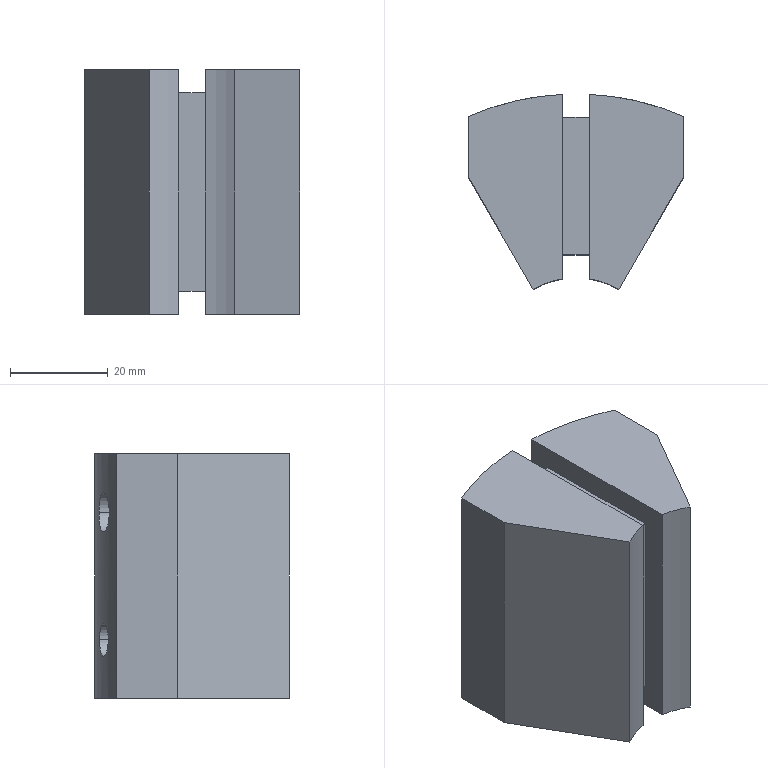Part | SolidWorks | features 3DProfileFeature 2, HoleWzd 2, Extrusion 1, ICE 1 | 1 solid | 34 faces | box 44 x 39.776 x 50 mm | volume 60767 mm3 | plane 14 | cylinder 12 | cone 8 | commonest cylinder face diameters 6.8 x4 8 x4 35 x2 110 x2
STEP:
#1=CARTESIAN_POINT('',(-9.048,33.766,-13.));
#2=VERTEX_POINT('',#1);
#3=CARTESIAN_POINT('',(-12.86,34.859,-13.));
#4=VERTEX_POINT('',#3);
#5=CARTESIAN_POINT('',(-12.86,34.859,-13.));
#6=DIRECTION('',(-0.9613,0.2756,0.));
#7=VECTOR('',#6,1000.);
#8=LINE('',#5,#7);
#9=EDGE_CURVE('',#2,#4,#8,.T.);
#10=ORIENTED_EDGE('',*,*,#9,.F.);
#11=CARTESIAN_POINT('',(-6.292,36.619,-13.));
#12=VERTEX_POINT('',#11);
#13=CARTESIAN_POINT('',(-6.292,36.619,-13.));
#14=DIRECTION('',(0.6947,0.7193,0.));
#15=VECTOR('',#14,1000.);
#16=LINE('',#13,#15);
#17=EDGE_CURVE('',#2,#12,#16,.T.);
#18=ORIENTED_EDGE('',*,*,#17,.T.);
#19=CARTESIAN_POINT('',(-9.576,35.739,-13.));
#20=DIRECTION('',(-0.2588,0.9659,0.));
#21=DIRECTION('',(-0.9659,-0.2588,0.));
#22=AXIS2_PLACEMENT_3D('',#19,#20,#21);
#23=CIRCLE('',#22,3.4);
#24=EDGE_CURVE('',#12,#4,#23,.T.);
#25=ORIENTED_EDGE('',*,*,#24,.T.);
#26=EDGE_LOOP('',(#10,#18,#25));
#27=FACE_OUTER_BOUND('',#26,.T.);
#28=CARTESIAN_POINT('',(-9.576,35.739,-13.));
#29=DIRECTION('',(-0.2588,0.9659,0.));
#30=DIRECTION('',(-0.9659,-0.2588,0.));
#31=AXIS2_PLACEMENT_3D('',#28,#29,#30);
#32=CONICAL_SURFACE('',#31,3.4,1.03);
#33=ADVANCED_FACE('',(#27),#32,.F.);
#34=ORIENTED_EDGE('',*,*,#24,.F.);
#35=CARTESIAN_POINT('',(-10.924,53.904,-13.));
#36=VERTEX_POINT('',#35);
#37=CARTESIAN_POINT('',(-10.951,54.006,-13.));
#38=DIRECTION('',(-0.2588,0.9659,0.));
#39=VECTOR('',#38,1000.);
#40=LINE('',#37,#39);
#41=EDGE_CURVE('',#12,#36,#40,.T.);
#42=ORIENTED_EDGE('',*,*,#41,.T.);
#43=CARTESIAN_POINT('',(-17.492,52.144,-13.));
#44=VERTEX_POINT('',#43);
#45=CARTESIAN_POINT('',(-17.492,52.144,-13.));
#46=CARTESIAN_POINT('',(-17.492,52.144,-13.225));
#47=CARTESIAN_POINT('',(-17.471,52.151,-13.446));
#48=CARTESIAN_POINT('',(-17.389,52.179,-13.88));
#49=CARTESIAN_POINT('',(-17.327,52.2,-14.096));
#50=CARTESIAN_POINT('',(-17.164,52.253,-14.508));
#51=CARTESIAN_POINT('',(-17.065,52.286,-14.703));
#52=CARTESIAN_POINT('',(-16.83,52.362,-15.073));
#53=CARTESIAN_POINT('',(-16.693,52.406,-15.248));
#54=CARTESIAN_POINT('',(-16.394,52.5,-15.561));
#55=CARTESIAN_POINT('',(-16.23,52.551,-15.702));
#56=CARTESIAN_POINT('',(-15.874,52.66,-15.951));
#57=CARTESIAN_POINT('',(-15.685,52.717,-16.056));
#58=CARTESIAN_POINT('',(-15.292,52.832,-16.226));
#59=CARTESIAN_POINT('',(-15.086,52.891,-16.291));
#60=CARTESIAN_POINT('',(-14.663,53.01,-16.378));
#61=CARTESIAN_POINT('',(-14.45,53.068,-16.4));
#62=CARTESIAN_POINT('',(-14.022,53.183,-16.4));
#63=CARTESIAN_POINT('',(-13.804,53.24,-16.378));
#64=CARTESIAN_POINT('',(-13.381,53.348,-16.291));
#65=CARTESIAN_POINT('',(-13.176,53.399,-16.227));
#66=CARTESIAN_POINT('',(-12.775,53.496,-16.057));
#67=CARTESIAN_POINT('',(-12.582,53.542,-15.95));
#68=CARTESIAN_POINT('',(-12.222,53.625,-15.704));
#69=CARTESIAN_POINT('',(-12.055,53.663,-15.563));
#70=CARTESIAN_POINT('',(-11.745,53.732,-15.246));
#71=CARTESIAN_POINT('',(-11.607,53.761,-15.074));
#72=CARTESIAN_POINT('',(-11.366,53.813,-14.706));
#73=CARTESIAN_POINT('',(-11.261,53.835,-14.507));
#74=CARTESIAN_POINT('',(-11.094,53.87,-14.095));
#75=CARTESIAN_POINT('',(-11.031,53.882,-13.883));
#76=CARTESIAN_POINT('',(-10.946,53.9,-13.447));
#77=CARTESIAN_POINT('',(-10.924,53.904,-13.222));
#78=CARTESIAN_POINT('',(-10.924,53.904,-13.));
#79=B_SPLINE_CURVE_WITH_KNOTS('',3,(#45,#46,#47,#48,#49,#50,#51,#52,#53,#54,#55,#56,#57,#58,#59,#60,#61,#62,#63,#64,#65,#66,#67,#68,#69,#70,#71,#72,#73,#74,#75,#76,#77,#78),.UNSPECIFIED.,.F.,.F.,(4,2,2,2,2,2,2,2,2,2,2,2,2,2,2,2,4),(0.,0.0006645,0.001329,0.001994,0.002658,0.003323,0.003987,0.004652,0.005316,0.005981,0.006645,0.00731,0.007974,0.008639,0.009303,0.009968,0.01063),.UNSPECIFIED.);
#80=EDGE_CURVE('',#44,#36,#79,.T.);
#81=ORIENTED_EDGE('',*,*,#80,.F.);
#82=CARTESIAN_POINT('',(-17.519,52.246,-13.));
#83=DIRECTION('',(-0.2588,0.9659,0.));
#84=VECTOR('',#83,1000.);
#85=LINE('',#82,#84);
#86=EDGE_CURVE('',#4,#44,#85,.T.);
#87=ORIENTED_EDGE('',*,*,#86,.F.);
#88=EDGE_LOOP('',(#34,#42,#81,#87));
#89=FACE_OUTER_BOUND('',#88,.T.);
#90=CARTESIAN_POINT('',(-14.235,53.126,-13.));
#91=DIRECTION('',(-0.2588,0.9659,0.));
#92=DIRECTION('',(-0.9659,-0.2588,0.));
#93=AXIS2_PLACEMENT_3D('',#90,#91,#92);
#94=CYLINDRICAL_SURFACE('',#93,3.4);
#95=ADVANCED_FACE('',(#89),#94,.F.);
#96=CARTESIAN_POINT('',(9.048,33.766,13.));
#97=VERTEX_POINT('',#96);
#98=CARTESIAN_POINT('',(6.292,36.619,13.));
#99=VERTEX_POINT('',#98);
#100=CARTESIAN_POINT('',(6.292,36.619,13.));
#101=DIRECTION('',(-0.6947,0.7193,0.));
#102=VECTOR('',#101,1000.);
#103=LINE('',#100,#102);
#104=EDGE_CURVE('',#97,#99,#103,.T.);
#105=ORIENTED_EDGE('',*,*,#104,.F.);
#106=CARTESIAN_POINT('',(12.86,34.859,13.));
#107=VERTEX_POINT('',#106);
#108=CARTESIAN_POINT('',(12.86,34.859,13.));
#109=DIRECTION('',(0.9613,0.2756,0.));
#110=VECTOR('',#109,1000.);
#111=LINE('',#108,#110);
#112=EDGE_CURVE('',#97,#107,#111,.T.);
#113=ORIENTED_EDGE('',*,*,#112,.T.);
#114=CARTESIAN_POINT('',(9.576,35.739,13.));
#115=DIRECTION('',(0.2588,0.9659,0.));
#116=DIRECTION('',(-0.9659,0.2588,0.));
#117=AXIS2_PLACEMENT_3D('',#114,#115,#116);
#118=CIRCLE('',#117,3.4);
#119=EDGE_CURVE('',#107,#99,#118,.T.);
#120=ORIENTED_EDGE('',*,*,#119,.T.);
#121=EDGE_LOOP('',(#105,#113,#120));
#122=FACE_OUTER_BOUND('',#121,.T.);
#123=CARTESIAN_POINT('',(9.576,35.739,13.));
#124=DIRECTION('',(0.2588,0.9659,0.));
#125=DIRECTION('',(-0.9659,0.2588,0.));
#126=AXIS2_PLACEMENT_3D('',#123,#124,#125);
#127=CONICAL_SURFACE('',#126,3.4,1.03);
#128=ADVANCED_FACE('',(#122),#127,.F.);
#129=ORIENTED_EDGE('',*,*,#119,.F.);
#130=CARTESIAN_POINT('',(17.492,52.144,13.));
#131=VERTEX_POINT('',#130);
#132=CARTESIAN_POINT('',(17.519,52.246,13.));
#133=DIRECTION('',(0.2588,0.9659,0.));
#134=VECTOR('',#133,1000.);
#135=LINE('',#132,#134);
#136=EDGE_CURVE('',#107,#131,#135,.T.);
#137=ORIENTED_EDGE('',*,*,#136,.T.);
#138=CARTESIAN_POINT('',(10.924,53.904,13.));
#139=VERTEX_POINT('',#138);
#140=CARTESIAN_POINT('',(10.924,53.904,13.));
#141=CARTESIAN_POINT('',(10.924,53.904,12.775));
#142=CARTESIAN_POINT('',(10.945,53.9,12.554));
#143=CARTESIAN_POINT('',(11.03,53.883,12.12));
#144=CARTESIAN_POINT('',(11.094,53.869,11.904));
#145=CARTESIAN_POINT('',(11.262,53.835,11.492));
#146=CARTESIAN_POINT('',(11.364,53.813,11.297));
#147=CARTESIAN_POINT('',(11.606,53.762,10.927));
#148=CARTESIAN_POINT('',(11.746,53.731,10.752));
#149=CARTESIAN_POINT('',(12.053,53.663,10.439));
#150=CARTESIAN_POINT('',(12.22,53.626,10.298));
#151=CARTESIAN_POINT('',(12.582,53.542,10.049));
#152=CARTESIAN_POINT('',(12.775,53.496,9.944));
#153=CARTESIAN_POINT('',(13.173,53.4,9.774));
#154=CARTESIAN_POINT('',(13.381,53.348,9.709));
#155=CARTESIAN_POINT('',(13.806,53.239,9.622));
#156=CARTESIAN_POINT('',(14.02,53.184,9.6));
#157=CARTESIAN_POINT('',(14.448,53.069,9.6));
#158=CARTESIAN_POINT('',(14.665,53.009,9.622));
#159=CARTESIAN_POINT('',(15.085,52.891,9.709));
#160=CARTESIAN_POINT('',(15.289,52.833,9.773));
#161=CARTESIAN_POINT('',(15.684,52.717,9.943));
#162=CARTESIAN_POINT('',(15.875,52.659,10.05));
#163=CARTESIAN_POINT('',(16.228,52.552,10.296));
#164=CARTESIAN_POINT('',(16.392,52.501,10.437));
#165=CARTESIAN_POINT('',(16.695,52.405,10.754));
#166=CARTESIAN_POINT('',(16.829,52.362,10.926));
#167=CARTESIAN_POINT('',(17.064,52.286,11.294));
#168=CARTESIAN_POINT('',(17.165,52.253,11.493));
#169=CARTESIAN_POINT('',(17.327,52.199,11.905));
#170=CARTESIAN_POINT('',(17.388,52.179,12.117));
#171=CARTESIAN_POINT('',(17.471,52.151,12.553));
#172=CARTESIAN_POINT('',(17.492,52.144,12.778));
#173=CARTESIAN_POINT('',(17.492,52.144,13.));
#174=B_SPLINE_CURVE_WITH_KNOTS('',3,(#140,#141,#142,#143,#144,#145,#146,#147,#148,#149,#150,#151,#152,#153,#154,#155,#156,#157,#158,#159,#160,#161,#162,#163,#164,#165,#166,#167,#168,#169,#170,#171,#172,#173),.UNSPECIFIED.,.F.,.F.,(4,2,2,2,2,2,2,2,2,2,2,2,2,2,2,2,4),(0.,0.0006645,0.001329,0.001994,0.002658,0.003323,0.003987,0.004652,0.005316,0.005981,0.006645,0.00731,0.007974,0.008639,0.009303,0.009968,0.01063),.UNSPECIFIED.);
#175=EDGE_CURVE('',#139,#131,#174,.T.);
#176=ORIENTED_EDGE('',*,*,#175,.F.);
#177=CARTESIAN_POINT('',(10.951,54.006,13.));
#178=DIRECTION('',(0.2588,0.9659,0.));
#179=VECTOR('',#178,1000.);
#180=LINE('',#177,#179);
#181=EDGE_CURVE('',#99,#139,#180,.T.);
#182=ORIENTED_EDGE('',*,*,#181,.F.);
#183=EDGE_LOOP('',(#129,#137,#176,#182));
#184=FACE_OUTER_BOUND('',#183,.T.);
#185=CARTESIAN_POINT('',(14.235,53.126,13.));
#186=DIRECTION('',(0.2588,0.9659,0.));
#187=DIRECTION('',(-0.9659,0.2588,0.));
#188=AXIS2_PLACEMENT_3D('',#185,#186,#187);
#189=CYLINDRICAL_SURFACE('',#188,3.4);
#190=ADVANCED_FACE('',(#184),#189,.F.);
#191=CARTESIAN_POINT('',(-9.731,36.315,13.));
#192=VERTEX_POINT('',#191);
#193=CARTESIAN_POINT('',(-14.216,37.602,13.));
#194=VERTEX_POINT('',#193);
#195=CARTESIAN_POINT('',(-14.216,37.602,13.));
#196=DIRECTION('',(-0.9613,0.2756,0.));
#197=VECTOR('',#196,1000.);
#198=LINE('',#195,#197);
#199=EDGE_CURVE('',#192,#194,#198,.T.);
#200=ORIENTED_EDGE('',*,*,#199,.F.);
#201=CARTESIAN_POINT('',(-6.489,39.672,13.));
#202=VERTEX_POINT('',#201);
#203=CARTESIAN_POINT('',(-6.489,39.672,13.));
#204=DIRECTION('',(0.6947,0.7193,0.));
#205=VECTOR('',#204,1000.);
#206=LINE('',#203,#205);
#207=EDGE_CURVE('',#192,#202,#206,.T.);
#208=ORIENTED_EDGE('',*,*,#207,.T.);
#209=CARTESIAN_POINT('',(-10.353,38.637,13.));
#210=DIRECTION('',(-0.2588,0.9659,0.));
#211=DIRECTION('',(-0.9659,-0.2588,0.));
#212=AXIS2_PLACEMENT_3D('',#209,#210,#211);
#213=CIRCLE('',#212,4.);
#214=EDGE_CURVE('',#202,#194,#213,.T.);
#215=ORIENTED_EDGE('',*,*,#214,.T.);
#216=EDGE_LOOP('',(#200,#208,#215));
#217=FACE_OUTER_BOUND('',#216,.T.);
#218=CARTESIAN_POINT('',(-10.353,38.637,13.));
#219=DIRECTION('',(-0.2588,0.9659,0.));
#220=DIRECTION('',(-0.9659,-0.2588,0.));
#221=AXIS2_PLACEMENT_3D('',#218,#219,#220);
#222=CONICAL_SURFACE('',#221,4.,1.03);
#223=ADVANCED_FACE('',(#217),#222,.F.);
#224=ORIENTED_EDGE('',*,*,#214,.F.);
#225=CARTESIAN_POINT('',(-10.334,54.021,13.));
#226=VERTEX_POINT('',#225);
#227=CARTESIAN_POINT('',(-10.371,54.161,13.));
#228=DIRECTION('',(-0.2588,0.9659,0.));
#229=VECTOR('',#228,1000.);
#230=LINE('',#227,#229);
#231=EDGE_CURVE('',#202,#226,#230,.T.);
#232=ORIENTED_EDGE('',*,*,#231,.T.);
#233=CARTESIAN_POINT('',(-18.061,51.95,13.));
#234=VERTEX_POINT('',#233);
#235=CARTESIAN_POINT('',(-18.061,51.95,13.));
#236=CARTESIAN_POINT('',(-18.061,51.95,12.736));
#237=CARTESIAN_POINT('',(-18.036,51.959,12.476));
#238=CARTESIAN_POINT('',(-17.94,51.992,11.964));
#239=CARTESIAN_POINT('',(-17.867,52.017,11.71));
#240=CARTESIAN_POINT('',(-17.677,52.082,11.226));
#241=CARTESIAN_POINT('',(-17.56,52.122,10.996));
#242=CARTESIAN_POINT('',(-17.284,52.214,10.561));
#243=CARTESIAN_POINT('',(-17.124,52.267,10.355));
#244=CARTESIAN_POINT('',(-16.772,52.381,9.987));
#245=CARTESIAN_POINT('',(-16.58,52.442,9.821));
#246=CARTESIAN_POINT('',(-16.162,52.572,9.529));
#247=CARTESIAN_POINT('',(-15.939,52.64,9.404));
#248=CARTESIAN_POINT('',(-15.478,52.778,9.205));
#249=CARTESIAN_POINT('',(-15.236,52.848,9.128));
#250=CARTESIAN_POINT('',(-14.739,52.989,9.025));
#251=CARTESIAN_POINT('',(-14.489,53.058,9.));
#252=CARTESIAN_POINT('',(-13.984,53.193,9.));
#253=CARTESIAN_POINT('',(-13.728,53.26,9.026));
#254=CARTESIAN_POINT('',(-13.23,53.386,9.128));
#255=CARTESIAN_POINT('',(-12.988,53.445,9.204));
#256=CARTESIAN_POINT('',(-12.517,53.557,9.404));
#257=CARTESIAN_POINT('',(-12.288,53.61,9.529));
#258=CARTESIAN_POINT('',(-11.865,53.705,9.819));
#259=CARTESIAN_POINT('',(-11.668,53.749,9.984));
#260=CARTESIAN_POINT('',(-11.302,53.827,10.358));
#261=CARTESIAN_POINT('',(-11.139,53.86,10.56));
#262=CARTESIAN_POINT('',(-10.855,53.918,10.993));
#263=CARTESIAN_POINT('',(-10.732,53.943,11.227));
#264=CARTESIAN_POINT('',(-10.535,53.982,11.712));
#265=CARTESIAN_POINT('',(-10.46,53.996,11.961));
#266=CARTESIAN_POINT('',(-10.359,54.016,12.474));
#267=CARTESIAN_POINT('',(-10.334,54.021,12.739));
#268=CARTESIAN_POINT('',(-10.334,54.021,13.));
#269=B_SPLINE_CURVE_WITH_KNOTS('',3,(#235,#236,#237,#238,#239,#240,#241,#242,#243,#244,#245,#246,#247,#248,#249,#250,#251,#252,#253,#254,#255,#256,#257,#258,#259,#260,#261,#262,#263,#264,#265,#266,#267,#268),.UNSPECIFIED.,.F.,.F.,(4,2,2,2,2,2,2,2,2,2,2,2,2,2,2,2,4),(0.,0.0007819,0.001564,0.002346,0.003127,0.003909,0.004691,0.005473,0.006255,0.007037,0.007819,0.008601,0.009382,0.01016,0.01095,0.01173,0.01251),.UNSPECIFIED.);
#270=EDGE_CURVE('',#234,#226,#269,.T.);
#271=ORIENTED_EDGE('',*,*,#270,.F.);
#272=CARTESIAN_POINT('',(-18.099,52.091,13.));
#273=DIRECTION('',(-0.2588,0.9659,0.));
#274=VECTOR('',#273,1000.);
#275=LINE('',#272,#274);
#276=EDGE_CURVE('',#194,#234,#275,.T.);
#277=ORIENTED_EDGE('',*,*,#276,.F.);
#278=EDGE_LOOP('',(#224,#232,#271,#277));
#279=FACE_OUTER_BOUND('',#278,.T.);
#280=CARTESIAN_POINT('',(-14.235,53.126,13.));
#281=DIRECTION('',(-0.2588,0.9659,0.));
#282=DIRECTION('',(-0.9659,-0.2588,0.));
#283=AXIS2_PLACEMENT_3D('',#280,#281,#282);
#284=CYLINDRICAL_SURFACE('',#283,4.);
#285=ADVANCED_FACE('',(#279),#284,.F.);
#286=CARTESIAN_POINT('',(9.731,36.315,-13.));
#287=VERTEX_POINT('',#286);
#288=CARTESIAN_POINT('',(6.489,39.672,-13.));
#289=VERTEX_POINT('',#288);
#290=CARTESIAN_POINT('',(6.489,39.672,-13.));
#291=DIRECTION('',(-0.6947,0.7193,0.));
#292=VECTOR('',#291,1000.);
#293=LINE('',#290,#292);
#294=EDGE_CURVE('',#287,#289,#293,.T.);
#295=ORIENTED_EDGE('',*,*,#294,.F.);
#296=CARTESIAN_POINT('',(14.216,37.602,-13.));
#297=VERTEX_POINT('',#296);
#298=CARTESIAN_POINT('',(14.216,37.602,-13.));
#299=DIRECTION('',(0.9613,0.2756,0.));
#300=VECTOR('',#299,1000.);
#301=LINE('',#298,#300);
#302=EDGE_CURVE('',#287,#297,#301,.T.);
#303=ORIENTED_EDGE('',*,*,#302,.T.);
#304=CARTESIAN_POINT('',(10.353,38.637,-13.));
#305=DIRECTION('',(0.2588,0.9659,0.));
#306=DIRECTION('',(-0.9659,0.2588,0.));
#307=AXIS2_PLACEMENT_3D('',#304,#305,#306);
#308=CIRCLE('',#307,4.);
#309=EDGE_CURVE('',#297,#289,#308,.T.);
#310=ORIENTED_EDGE('',*,*,#309,.T.);
#311=EDGE_LOOP('',(#295,#303,#310));
#312=FACE_OUTER_BOUND('',#311,.T.);
#313=CARTESIAN_POINT('',(10.353,38.637,-13.));
#314=DIRECTION('',(0.2588,0.9659,0.));
#315=DIRECTION('',(-0.9659,0.2588,0.));
#316=AXIS2_PLACEMENT_3D('',#313,#314,#315);
#317=CONICAL_SURFACE('',#316,4.,1.03);
#318=ADVANCED_FACE('',(#312),#317,.F.);
#319=ORIENTED_EDGE('',*,*,#309,.F.);
#320=CARTESIAN_POINT('',(18.061,51.95,-13.));
#321=VERTEX_POINT('',#320);
#322=CARTESIAN_POINT('',(18.099,52.091,-13.));
#323=DIRECTION('',(0.2588,0.9659,0.));
#324=VECTOR('',#323,1000.);
#325=LINE('',#322,#324);
#326=EDGE_CURVE('',#297,#321,#325,.T.);
#327=ORIENTED_EDGE('',*,*,#326,.T.);
#328=CARTESIAN_POINT('',(10.334,54.021,-13.));
#329=VERTEX_POINT('',#328);
#330=CARTESIAN_POINT('',(10.334,54.021,-13.));
#331=CARTESIAN_POINT('',(10.334,54.021,-13.264));
#332=CARTESIAN_POINT('',(10.359,54.016,-13.524));
#333=CARTESIAN_POINT('',(10.459,53.996,-14.036));
#334=CARTESIAN_POINT('',(10.535,53.982,-14.29));
#335=CARTESIAN_POINT('',(10.733,53.943,-14.774));
#336=CARTESIAN_POINT('',(10.853,53.919,-15.004));
#337=CARTESIAN_POINT('',(11.138,53.861,-15.439));
#338=CARTESIAN_POINT('',(11.304,53.826,-15.645));
#339=CARTESIAN_POINT('',(11.665,53.749,-16.013));
#340=CARTESIAN_POINT('',(11.862,53.706,-16.179));
#341=CARTESIAN_POINT('',(12.289,53.61,-16.471));
#342=CARTESIAN_POINT('',(12.516,53.557,-16.596));
#343=CARTESIAN_POINT('',(12.985,53.446,-16.795));
#344=CARTESIAN_POINT('',(13.23,53.386,-16.872));
#345=CARTESIAN_POINT('',(13.73,53.259,-16.975));
#346=CARTESIAN_POINT('',(13.982,53.194,-17.));
#347=CARTESIAN_POINT('',(14.486,53.059,-17.));
#348=CARTESIAN_POINT('',(14.741,52.988,-16.974));
#349=CARTESIAN_POINT('',(15.235,52.848,-16.872));
#350=CARTESIAN_POINT('',(15.475,52.779,-16.796));
#351=CARTESIAN_POINT('',(15.939,52.64,-16.596));
#352=CARTESIAN_POINT('',(16.163,52.572,-16.471));
#353=CARTESIAN_POINT('',(16.577,52.443,-16.181));
#354=CARTESIAN_POINT('',(16.77,52.381,-16.016));
#355=CARTESIAN_POINT('',(17.126,52.266,-15.642));
#356=CARTESIAN_POINT('',(17.283,52.214,-15.44));
#357=CARTESIAN_POINT('',(17.558,52.122,-15.007));
#358=CARTESIAN_POINT('',(17.677,52.082,-14.773));
#359=CARTESIAN_POINT('',(17.868,52.017,-14.288));
#360=CARTESIAN_POINT('',(17.939,51.992,-14.039));
#361=CARTESIAN_POINT('',(18.036,51.959,-13.526));
#362=CARTESIAN_POINT('',(18.061,51.95,-13.261));
#363=CARTESIAN_POINT('',(18.061,51.95,-13.));
#364=B_SPLINE_CURVE_WITH_KNOTS('',3,(#330,#331,#332,#333,#334,#335,#336,#337,#338,#339,#340,#341,#342,#343,#344,#345,#346,#347,#348,#349,#350,#351,#352,#353,#354,#355,#356,#357,#358,#359,#360,#361,#362,#363),.UNSPECIFIED.,.F.,.F.,(4,2,2,2,2,2,2,2,2,2,2,2,2,2,2,2,4),(0.,0.0007819,0.001564,0.002346,0.003127,0.003909,0.004691,0.005473,0.006255,0.007037,0.007819,0.008601,0.009382,0.01016,0.01095,0.01173,0.01251),.UNSPECIFIED.);
#365=EDGE_CURVE('',#329,#321,#364,.T.);
#366=ORIENTED_EDGE('',*,*,#365,.F.);
#367=CARTESIAN_POINT('',(10.371,54.161,-13.));
#368=DIRECTION('',(0.2588,0.9659,0.));
#369=VECTOR('',#368,1000.);
#370=LINE('',#367,#369);
#371=EDGE_CURVE('',#289,#329,#370,.T.);
#372=ORIENTED_EDGE('',*,*,#371,.F.);
#373=EDGE_LOOP('',(#319,#327,#366,#372));
#374=FACE_OUTER_BOUND('',#373,.T.);
#375=CARTESIAN_POINT('',(14.235,53.126,-13.));
#376=DIRECTION('',(0.2588,0.9659,0.));
#377=DIRECTION('',(-0.9659,0.2588,0.));
#378=AXIS2_PLACEMENT_3D('',#375,#376,#377);
#379=CYLINDRICAL_SURFACE('',#378,4.);
#380=ADVANCED_FACE('',(#374),#379,.F.);
#381=CARTESIAN_POINT('',(-8.75,15.155,-25.));
#382=VERTEX_POINT('',#381);
#383=CARTESIAN_POINT('',(-2.75,17.283,-25.));
#384=VERTEX_POINT('',#383);
#385=CARTESIAN_POINT('',(0.,0.,-25.));
#386=DIRECTION('',(0.,0.,-1.));
#387=DIRECTION('',(1.,0.,0.));
#388=AXIS2_PLACEMENT_3D('',#385,#386,#387);
#389=CIRCLE('',#388,17.5);
#390=EDGE_CURVE('',#382,#384,#389,.T.);
#391=ORIENTED_EDGE('',*,*,#390,.T.);
#392=CARTESIAN_POINT('',(-2.75,17.283,25.));
#393=VERTEX_POINT('',#392);
#394=CARTESIAN_POINT('',(-2.75,17.283,25.));
#395=DIRECTION('',(0.,0.,-1.));
#396=VECTOR('',#395,1000.);
#397=LINE('',#394,#396);
#398=EDGE_CURVE('',#393,#384,#397,.T.);
#399=ORIENTED_EDGE('',*,*,#398,.F.);
#400=CARTESIAN_POINT('',(-8.75,15.155,25.));
#401=VERTEX_POINT('',#400);
#402=CARTESIAN_POINT('',(0.,0.,25.));
#403=DIRECTION('',(0.,0.,-1.));
#404=DIRECTION('',(1.,0.,0.));
#405=AXIS2_PLACEMENT_3D('',#402,#403,#404);
#406=CIRCLE('',#405,17.5);
#407=EDGE_CURVE('',#401,#393,#406,.T.);
#408=ORIENTED_EDGE('',*,*,#407,.F.);
#409=CARTESIAN_POINT('',(-8.75,15.155,25.));
#410=DIRECTION('',(0.,0.,-1.));
#411=VECTOR('',#410,1000.);
#412=LINE('',#409,#411);
#413=EDGE_CURVE('',#401,#382,#412,.T.);
#414=ORIENTED_EDGE('',*,*,#413,.T.);
#415=EDGE_LOOP('',(#391,#399,#408,#414));
#416=FACE_OUTER_BOUND('',#415,.T.);
#417=CARTESIAN_POINT('',(0.,0.,25.));
#418=DIRECTION('',(0.,0.,-1.));
#419=DIRECTION('',(-1.,0.,0.));
#420=AXIS2_PLACEMENT_3D('',#417,#418,#419);
#421=CYLINDRICAL_SURFACE('',#420,17.5);
#422=ADVANCED_FACE('',(#416),#421,.F.);
#423=CARTESIAN_POINT('',(-2.75,50.3,20.3));
#424=VERTEX_POINT('',#423);
#425=CARTESIAN_POINT('',(-2.75,50.3,-20.3));
#426=VERTEX_POINT('',#425);
#427=CARTESIAN_POINT('',(-2.75,50.3,20.3));
#428=DIRECTION('',(0.,0.,-1.));
#429=VECTOR('',#428,1000.);
#430=LINE('',#427,#429);
#431=EDGE_CURVE('',#424,#426,#430,.T.);
#432=ORIENTED_EDGE('',*,*,#431,.T.);
#433=CARTESIAN_POINT('',(-2.75,22.2,-20.3));
#434=VERTEX_POINT('',#433);
#435=CARTESIAN_POINT('',(-2.75,22.2,-20.3));
#436=DIRECTION('',(0.,-1.,0.));
#437=VECTOR('',#436,1000.);
#438=LINE('',#435,#437);
#439=EDGE_CURVE('',#426,#434,#438,.T.);
#440=ORIENTED_EDGE('',*,*,#439,.T.);
#441=CARTESIAN_POINT('',(-2.75,22.2,20.3));
#442=VERTEX_POINT('',#441);
#443=CARTESIAN_POINT('',(-2.75,22.2,20.3));
#444=DIRECTION('',(0.,0.,-1.));
#445=VECTOR('',#444,1000.);
#446=LINE('',#443,#445);
#447=EDGE_CURVE('',#442,#434,#446,.T.);
#448=ORIENTED_EDGE('',*,*,#447,.F.);
#449=CARTESIAN_POINT('',(-2.75,22.2,20.3));
#450=DIRECTION('',(0.,-1.,0.));
#451=VECTOR('',#450,1000.);
#452=LINE('',#449,#451);
#453=EDGE_CURVE('',#424,#442,#452,.T.);
#454=ORIENTED_EDGE('',*,*,#453,.F.);
#455=EDGE_LOOP('',(#432,#440,#448,#454));
#456=FACE_BOUND('',#455,.T.);
#457=CARTESIAN_POINT('',(-2.75,54.931,-25.));
#458=VERTEX_POINT('',#457);
#459=CARTESIAN_POINT('',(-2.75,54.931,-25.));
#460=DIRECTION('',(0.,1.,0.));
#461=VECTOR('',#460,1000.);
#462=LINE('',#459,#461);
#463=EDGE_CURVE('',#384,#458,#462,.T.);
#464=ORIENTED_EDGE('',*,*,#463,.T.);
#465=CARTESIAN_POINT('',(-2.75,54.931,25.));
#466=VERTEX_POINT('',#465);
#467=CARTESIAN_POINT('',(-2.75,54.931,25.));
#468=DIRECTION('',(0.,0.,-1.));
#469=VECTOR('',#468,1000.);
#470=LINE('',#467,#469);
#471=EDGE_CURVE('',#466,#458,#470,.T.);
#472=ORIENTED_EDGE('',*,*,#471,.F.);
#473=CARTESIAN_POINT('',(-2.75,54.931,25.));
#474=DIRECTION('',(0.,1.,0.));
#475=VECTOR('',#474,1000.);
#476=LINE('',#473,#475);
#477=EDGE_CURVE('',#393,#466,#476,.T.);
#478=ORIENTED_EDGE('',*,*,#477,.F.);
#479=ORIENTED_EDGE('',*,*,#398,.T.);
#480=EDGE_LOOP('',(#464,#472,#478,#479));
#481=FACE_OUTER_BOUND('',#480,.T.);
#482=CARTESIAN_POINT('',(-2.75,54.931,25.));
#483=DIRECTION('',(-1.,0.,0.));
#484=DIRECTION('',(0.,-1.,0.));
#485=AXIS2_PLACEMENT_3D('',#482,#483,#484);
#486=PLANE('',#485);
#487=ADVANCED_FACE('',(#456,#481),#486,.F.);
#488=ORIENTED_EDGE('',*,*,#80,.T.);
#489=CARTESIAN_POINT('',(-10.924,53.904,-13.));
#490=CARTESIAN_POINT('',(-10.924,53.904,-12.778));
#491=CARTESIAN_POINT('',(-10.945,53.9,-12.558));
#492=CARTESIAN_POINT('',(-11.03,53.883,-12.119));
#493=CARTESIAN_POINT('',(-11.094,53.87,-11.904));
#494=CARTESIAN_POINT('',(-11.26,53.835,-11.495));
#495=CARTESIAN_POINT('',(-11.363,53.813,-11.298));
#496=CARTESIAN_POINT('',(-11.607,53.761,-10.926));
#497=CARTESIAN_POINT('',(-11.745,53.732,-10.754));
#498=CARTESIAN_POINT('',(-12.051,53.664,-10.441));
#499=CARTESIAN_POINT('',(-12.221,53.625,-10.297));
#500=CARTESIAN_POINT('',(-12.581,53.542,-10.05));
#501=CARTESIAN_POINT('',(-12.771,53.497,-9.945));
#502=CARTESIAN_POINT('',(-13.171,53.4,-9.775));
#503=CARTESIAN_POINT('',(-13.381,53.348,-9.709));
#504=CARTESIAN_POINT('',(-13.802,53.24,-9.622));
#505=CARTESIAN_POINT('',(-14.016,53.185,-9.6));
#506=CARTESIAN_POINT('',(-14.449,53.069,-9.6));
#507=CARTESIAN_POINT('',(-14.663,53.01,-9.622));
#508=CARTESIAN_POINT('',(-15.081,52.892,-9.708));
#509=CARTESIAN_POINT('',(-15.288,52.833,-9.773));
#510=CARTESIAN_POINT('',(-15.684,52.717,-9.943));
#511=CARTESIAN_POINT('',(-15.871,52.661,-10.048));
#512=CARTESIAN_POINT('',(-16.225,52.553,-10.294));
#513=CARTESIAN_POINT('',(-16.392,52.501,-10.437));
#514=CARTESIAN_POINT('',(-16.692,52.406,-10.751));
#515=CARTESIAN_POINT('',(-16.826,52.363,-10.922));
#516=CARTESIAN_POINT('',(-17.063,52.286,-11.293));
#517=CARTESIAN_POINT('',(-17.164,52.253,-11.491));
#518=CARTESIAN_POINT('',(-17.406,52.173,-12.104));
#519=CARTESIAN_POINT('',(-17.492,52.144,-12.551));
#520=CARTESIAN_POINT('',(-17.492,52.144,-13.));
#521=B_SPLINE_CURVE_WITH_KNOTS('',3,(#489,#490,#491,#492,#493,#494,#495,#496,#497,#498,#499,#500,#501,#502,#503,#504,#505,#506,#507,#508,#509,#510,#511,#512,#513,#514,#515,#516,#517,#518,#519,#520),.UNSPECIFIED.,.F.,.F.,(4,2,2,2,2,2,2,2,2,2,2,2,2,2,2,4),(0.01063,0.0113,0.01196,0.01263,0.01329,0.01395,0.01462,0.01528,0.01595,0.01661,0.01728,0.01794,0.01861,0.01927,0.01993,0.02126),.UNSPECIFIED.);
#522=EDGE_CURVE('',#36,#44,#521,.T.);
#523=ORIENTED_EDGE('',*,*,#522,.T.);
#524=EDGE_LOOP('',(#488,#523));
#525=FACE_BOUND('',#524,.T.);
#526=ORIENTED_EDGE('',*,*,#270,.T.);
#527=CARTESIAN_POINT('',(-10.334,54.021,13.));
#528=CARTESIAN_POINT('',(-10.334,54.021,13.261));
#529=CARTESIAN_POINT('',(-10.359,54.016,13.521));
#530=CARTESIAN_POINT('',(-10.459,53.996,14.036));
#531=CARTESIAN_POINT('',(-10.535,53.982,14.289));
#532=CARTESIAN_POINT('',(-10.731,53.943,14.77));
#533=CARTESIAN_POINT('',(-10.853,53.919,15.003));
#534=CARTESIAN_POINT('',(-11.14,53.86,15.441));
#535=CARTESIAN_POINT('',(-11.302,53.827,15.642));
#536=CARTESIAN_POINT('',(-11.663,53.75,16.011));
#537=CARTESIAN_POINT('',(-11.864,53.706,16.18));
#538=CARTESIAN_POINT('',(-12.288,53.61,16.471));
#539=CARTESIAN_POINT('',(-12.512,53.558,16.594));
#540=CARTESIAN_POINT('',(-12.983,53.446,16.794));
#541=CARTESIAN_POINT('',(-13.23,53.386,16.872));
#542=CARTESIAN_POINT('',(-13.726,53.26,16.974));
#543=CARTESIAN_POINT('',(-13.977,53.195,17.));
#544=CARTESIAN_POINT('',(-14.487,53.058,17.));
#545=CARTESIAN_POINT('',(-14.738,52.989,16.974));
#546=CARTESIAN_POINT('',(-15.23,52.85,16.873));
#547=CARTESIAN_POINT('',(-15.474,52.779,16.797));
#548=CARTESIAN_POINT('',(-15.939,52.64,16.596));
#549=CARTESIAN_POINT('',(-16.159,52.573,16.473));
#550=CARTESIAN_POINT('',(-16.574,52.444,16.184));
#551=CARTESIAN_POINT('',(-16.77,52.381,16.015));
#552=CARTESIAN_POINT('',(-17.122,52.267,15.646));
#553=CARTESIAN_POINT('',(-17.28,52.215,15.445));
#554=CARTESIAN_POINT('',(-17.558,52.122,15.008));
#555=CARTESIAN_POINT('',(-17.676,52.082,14.775));
#556=CARTESIAN_POINT('',(-17.866,52.018,14.294));
#557=CARTESIAN_POINT('',(-17.938,51.992,14.043));
#558=CARTESIAN_POINT('',(-18.036,51.959,13.526));
#559=CARTESIAN_POINT('',(-18.061,51.95,13.264));
#560=CARTESIAN_POINT('',(-18.061,51.95,13.));
#561=B_SPLINE_CURVE_WITH_KNOTS('',3,(#527,#528,#529,#530,#531,#532,#533,#534,#535,#536,#537,#538,#539,#540,#541,#542,#543,#544,#545,#546,#547,#548,#549,#550,#551,#552,#553,#554,#555,#556,#557,#558,#559,#560),.UNSPECIFIED.,.F.,.F.,(4,2,2,2,2,2,2,2,2,2,2,2,2,2,2,2,4),(0.01251,0.01329,0.01407,0.01486,0.01564,0.01642,0.0172,0.01798,0.01876,0.01955,0.02033,0.02111,0.02189,0.02267,0.02345,0.02424,0.02502),.UNSPECIFIED.);
#562=EDGE_CURVE('',#226,#234,#561,.T.);
#563=ORIENTED_EDGE('',*,*,#562,.T.);
#564=EDGE_LOOP('',(#526,#563));
#565=FACE_BOUND('',#564,.T.);
#566=CARTESIAN_POINT('',(-22.,50.408,-25.));
#567=VERTEX_POINT('',#566);
#568=CARTESIAN_POINT('',(0.,0.,-25.));
#569=DIRECTION('',(0.,0.,1.));
#570=DIRECTION('',(1.,0.,0.));
#571=AXIS2_PLACEMENT_3D('',#568,#569,#570);
#572=CIRCLE('',#571,55.);
#573=EDGE_CURVE('',#458,#567,#572,.T.);
#574=ORIENTED_EDGE('',*,*,#573,.T.);
#575=CARTESIAN_POINT('',(-22.,50.408,25.));
#576=VERTEX_POINT('',#575);
#577=CARTESIAN_POINT('',(-22.,50.408,25.));
#578=DIRECTION('',(0.,0.,-1.));
#579=VECTOR('',#578,1000.);
#580=LINE('',#577,#579);
#581=EDGE_CURVE('',#576,#567,#580,.T.);
#582=ORIENTED_EDGE('',*,*,#581,.F.);
#583=CARTESIAN_POINT('',(0.,0.,25.));
#584=DIRECTION('',(0.,0.,1.));
#585=DIRECTION('',(1.,0.,0.));
#586=AXIS2_PLACEMENT_3D('',#583,#584,#585);
#587=CIRCLE('',#586,55.);
#588=EDGE_CURVE('',#466,#576,#587,.T.);
#589=ORIENTED_EDGE('',*,*,#588,.F.);
#590=ORIENTED_EDGE('',*,*,#471,.T.);
#591=EDGE_LOOP('',(#574,#582,#589,#590));
#592=FACE_OUTER_BOUND('',#591,.T.);
#593=CARTESIAN_POINT('',(0.,0.,25.));
#594=DIRECTION('',(0.,0.,-1.));
#595=DIRECTION('',(-1.,0.,0.));
#596=AXIS2_PLACEMENT_3D('',#593,#594,#595);
#597=CYLINDRICAL_SURFACE('',#596,55.);
#598=ADVANCED_FACE('',(#525,#565,#592),#597,.T.);
#599=CARTESIAN_POINT('',(-22.,38.105,-25.));
#600=VERTEX_POINT('',#599);
#601=CARTESIAN_POINT('',(-22.,50.408,-25.));
#602=DIRECTION('',(0.,-1.,0.));
#603=VECTOR('',#602,1000.);
#604=LINE('',#601,#603);
#605=EDGE_CURVE('',#567,#600,#604,.T.);
#606=ORIENTED_EDGE('',*,*,#605,.T.);
#607=CARTESIAN_POINT('',(-22.,38.105,25.));
#608=VERTEX_POINT('',#607);
#609=CARTESIAN_POINT('',(-22.,38.105,25.));
#610=DIRECTION('',(0.,0.,-1.));
#611=VECTOR('',#610,1000.);
#612=LINE('',#609,#611);
#613=EDGE_CURVE('',#608,#600,#612,.T.);
#614=ORIENTED_EDGE('',*,*,#613,.F.);
#615=CARTESIAN_POINT('',(-22.,50.408,25.));
#616=DIRECTION('',(0.,-1.,0.));
#617=VECTOR('',#616,1000.);
#618=LINE('',#615,#617);
#619=EDGE_CURVE('',#576,#608,#618,.T.);
#620=ORIENTED_EDGE('',*,*,#619,.F.);
#621=ORIENTED_EDGE('',*,*,#581,.T.);
#622=EDGE_LOOP('',(#606,#614,#620,#621));
#623=FACE_OUTER_BOUND('',#622,.T.);
#624=CARTESIAN_POINT('',(-22.,50.408,25.));
#625=DIRECTION('',(1.,0.,0.));
#626=DIRECTION('',(0.,0.,-1.));
#627=AXIS2_PLACEMENT_3D('',#624,#625,#626);
#628=PLANE('',#627);
#629=ADVANCED_FACE('',(#623),#628,.F.);
#630=CARTESIAN_POINT('',(-8.75,15.155,-25.));
#631=DIRECTION('',(0.5,-0.866,0.));
#632=VECTOR('',#631,1000.);
#633=LINE('',#630,#632);
#634=EDGE_CURVE('',#600,#382,#633,.T.);
#635=ORIENTED_EDGE('',*,*,#634,.T.);
#636=ORIENTED_EDGE('',*,*,#413,.F.);
#637=CARTESIAN_POINT('',(-8.75,15.155,25.));
#638=DIRECTION('',(0.5,-0.866,0.));
#639=VECTOR('',#638,1000.);
#640=LINE('',#637,#639);
#641=EDGE_CURVE('',#608,#401,#640,.T.);
#642=ORIENTED_EDGE('',*,*,#641,.F.);
#643=ORIENTED_EDGE('',*,*,#613,.T.);
#644=EDGE_LOOP('',(#635,#636,#642,#643));
#645=FACE_OUTER_BOUND('',#644,.T.);
#646=CARTESIAN_POINT('',(-8.75,15.155,25.));
#647=DIRECTION('',(0.866,0.5,0.));
#648=DIRECTION('',(-0.5,0.866,0.));
#649=AXIS2_PLACEMENT_3D('',#646,#647,#648);
#650=PLANE('',#649);
#651=ADVANCED_FACE('',(#645),#650,.F.);
#652=ORIENTED_EDGE('',*,*,#407,.T.);
#653=ORIENTED_EDGE('',*,*,#477,.T.);
#654=ORIENTED_EDGE('',*,*,#588,.T.);
#655=ORIENTED_EDGE('',*,*,#619,.T.);
#656=ORIENTED_EDGE('',*,*,#641,.T.);
#657=EDGE_LOOP('',(#652,#653,#654,#655,#656));
#658=FACE_OUTER_BOUND('',#657,.T.);
#659=CARTESIAN_POINT('',(0.,0.,25.));
#660=DIRECTION('',(0.,0.,1.));
#661=DIRECTION('',(1.,0.,0.));
#662=AXIS2_PLACEMENT_3D('',#659,#660,#661);
#663=PLANE('',#662);
#664=ADVANCED_FACE('',(#658),#663,.T.);
#665=ORIENTED_EDGE('',*,*,#390,.F.);
#666=ORIENTED_EDGE('',*,*,#634,.F.);
#667=ORIENTED_EDGE('',*,*,#605,.F.);
#668=ORIENTED_EDGE('',*,*,#573,.F.);
#669=ORIENTED_EDGE('',*,*,#463,.F.);
#670=EDGE_LOOP('',(#665,#666,#667,#668,#669));
#671=FACE_OUTER_BOUND('',#670,.T.);
#672=CARTESIAN_POINT('',(0.,0.,-25.));
#673=DIRECTION('',(0.,0.,1.));
#674=DIRECTION('',(1.,0.,0.));
#675=AXIS2_PLACEMENT_3D('',#672,#673,#674);
#676=PLANE('',#675);
#677=ADVANCED_FACE('',(#671),#676,.F.);
#678=CARTESIAN_POINT('',(2.75,22.2,-20.3));
#679=VERTEX_POINT('',#678);
#680=CARTESIAN_POINT('',(2.75,22.2,-20.3));
#681=DIRECTION('',(1.,0.,0.));
#682=VECTOR('',#681,1000.);
#683=LINE('',#680,#682);
#684=EDGE_CURVE('',#434,#679,#683,.T.);
#685=ORIENTED_EDGE('',*,*,#684,.T.);
#686=CARTESIAN_POINT('',(2.75,22.2,20.3));
#687=VERTEX_POINT('',#686);
#688=CARTESIAN_POINT('',(2.75,22.2,20.3));
#689=DIRECTION('',(0.,0.,-1.));
#690=VECTOR('',#689,1000.);
#691=LINE('',#688,#690);
#692=EDGE_CURVE('',#687,#679,#691,.T.);
#693=ORIENTED_EDGE('',*,*,#692,.F.);
#694=CARTESIAN_POINT('',(2.75,22.2,20.3));
#695=DIRECTION('',(1.,0.,0.));
#696=VECTOR('',#695,1000.);
#697=LINE('',#694,#696);
#698=EDGE_CURVE('',#442,#687,#697,.T.);
#699=ORIENTED_EDGE('',*,*,#698,.F.);
#700=ORIENTED_EDGE('',*,*,#447,.T.);
#701=EDGE_LOOP('',(#685,#693,#699,#700));
#702=FACE_OUTER_BOUND('',#701,.T.);
#703=CARTESIAN_POINT('',(2.75,22.2,20.3));
#704=DIRECTION('',(0.,1.,0.));
#705=DIRECTION('',(0.,0.,1.));
#706=AXIS2_PLACEMENT_3D('',#703,#704,#705);
#707=PLANE('',#706);
#708=ADVANCED_FACE('',(#702),#707,.F.);
#709=CARTESIAN_POINT('',(2.75,50.3,-20.3));
#710=VERTEX_POINT('',#709);
#711=CARTESIAN_POINT('',(2.75,50.3,-20.3));
#712=DIRECTION('',(-1.,0.,0.));
#713=VECTOR('',#712,1000.);
#714=LINE('',#711,#713);
#715=EDGE_CURVE('',#710,#426,#714,.T.);
#716=ORIENTED_EDGE('',*,*,#715,.T.);
#717=ORIENTED_EDGE('',*,*,#431,.F.);
#718=CARTESIAN_POINT('',(2.75,50.3,20.3));
#719=VERTEX_POINT('',#718);
#720=CARTESIAN_POINT('',(2.75,50.3,20.3));
#721=DIRECTION('',(-1.,0.,0.));
#722=VECTOR('',#721,1000.);
#723=LINE('',#720,#722);
#724=EDGE_CURVE('',#719,#424,#723,.T.);
#725=ORIENTED_EDGE('',*,*,#724,.F.);
#726=CARTESIAN_POINT('',(2.75,50.3,20.3));
#727=DIRECTION('',(0.,0.,-1.));
#728=VECTOR('',#727,1000.);
#729=LINE('',#726,#728);
#730=EDGE_CURVE('',#719,#710,#729,.T.);
#731=ORIENTED_EDGE('',*,*,#730,.T.);
#732=EDGE_LOOP('',(#716,#717,#725,#731));
#733=FACE_OUTER_BOUND('',#732,.T.);
#734=CARTESIAN_POINT('',(2.75,50.3,20.3));
#735=DIRECTION('',(0.,-1.,0.));
#736=DIRECTION('',(0.,0.,-1.));
#737=AXIS2_PLACEMENT_3D('',#734,#735,#736);
#738=PLANE('',#737);
#739=ADVANCED_FACE('',(#733),#738,.F.);
#740=ORIENTED_EDGE('',*,*,#453,.T.);
#741=ORIENTED_EDGE('',*,*,#698,.T.);
#742=CARTESIAN_POINT('',(2.75,22.2,20.3));
#743=DIRECTION('',(0.,1.,0.));
#744=VECTOR('',#743,1000.);
#745=LINE('',#742,#744);
#746=EDGE_CURVE('',#687,#719,#745,.T.);
#747=ORIENTED_EDGE('',*,*,#746,.T.);
#748=ORIENTED_EDGE('',*,*,#724,.T.);
#749=EDGE_LOOP('',(#740,#741,#747,#748));
#750=FACE_OUTER_BOUND('',#749,.T.);
#751=CARTESIAN_POINT('',(0.,0.,20.3));
#752=DIRECTION('',(0.,0.,1.));
#753=DIRECTION('',(1.,0.,0.));
#754=AXIS2_PLACEMENT_3D('',#751,#752,#753);
#755=PLANE('',#754);
#756=ADVANCED_FACE('',(#750),#755,.T.);
#757=ORIENTED_EDGE('',*,*,#439,.F.);
#758=ORIENTED_EDGE('',*,*,#715,.F.);
#759=CARTESIAN_POINT('',(2.75,22.2,-20.3));
#760=DIRECTION('',(0.,1.,0.));
#761=VECTOR('',#760,1000.);
#762=LINE('',#759,#761);
#763=EDGE_CURVE('',#679,#710,#762,.T.);
#764=ORIENTED_EDGE('',*,*,#763,.F.);
#765=ORIENTED_EDGE('',*,*,#684,.F.);
#766=EDGE_LOOP('',(#757,#758,#764,#765));
#767=FACE_OUTER_BOUND('',#766,.T.);
#768=CARTESIAN_POINT('',(0.,0.,-20.3));
#769=DIRECTION('',(0.,0.,1.));
#770=DIRECTION('',(1.,0.,0.));
#771=AXIS2_PLACEMENT_3D('',#768,#769,#770);
#772=PLANE('',#771);
#773=ADVANCED_FACE('',(#767),#772,.F.);
#774=CARTESIAN_POINT('',(2.75,54.931,-25.));
#775=VERTEX_POINT('',#774);
#776=CARTESIAN_POINT('',(2.75,17.283,-25.));
#777=VERTEX_POINT('',#776);
#778=CARTESIAN_POINT('',(2.75,54.931,-25.));
#779=DIRECTION('',(0.,-1.,0.));
#780=VECTOR('',#779,1000.);
#781=LINE('',#778,#780);
#782=EDGE_CURVE('',#775,#777,#781,.T.);
#783=ORIENTED_EDGE('',*,*,#782,.T.);
#784=CARTESIAN_POINT('',(2.75,17.283,25.));
#785=VERTEX_POINT('',#784);
#786=CARTESIAN_POINT('',(2.75,17.283,25.));
#787=DIRECTION('',(0.,0.,-1.));
#788=VECTOR('',#787,1000.);
#789=LINE('',#786,#788);
#790=EDGE_CURVE('',#785,#777,#789,.T.);
#791=ORIENTED_EDGE('',*,*,#790,.F.);
#792=CARTESIAN_POINT('',(2.75,54.931,25.));
#793=VERTEX_POINT('',#792);
#794=CARTESIAN_POINT('',(2.75,54.931,25.));
#795=DIRECTION('',(0.,-1.,0.));
#796=VECTOR('',#795,1000.);
#797=LINE('',#794,#796);
#798=EDGE_CURVE('',#793,#785,#797,.T.);
#799=ORIENTED_EDGE('',*,*,#798,.F.);
#800=CARTESIAN_POINT('',(2.75,54.931,25.));
#801=DIRECTION('',(0.,0.,-1.));
#802=VECTOR('',#801,1000.);
#803=LINE('',#800,#802);
#804=EDGE_CURVE('',#793,#775,#803,.T.);
#805=ORIENTED_EDGE('',*,*,#804,.T.);
#806=EDGE_LOOP('',(#783,#791,#799,#805));
#807=FACE_OUTER_BOUND('',#806,.T.);
#808=ORIENTED_EDGE('',*,*,#692,.T.);
#809=ORIENTED_EDGE('',*,*,#763,.T.);
#810=ORIENTED_EDGE('',*,*,#730,.F.);
#811=ORIENTED_EDGE('',*,*,#746,.F.);
#812=EDGE_LOOP('',(#808,#809,#810,#811));
#813=FACE_BOUND('',#812,.T.);
#814=CARTESIAN_POINT('',(2.75,54.931,25.));
#815=DIRECTION('',(1.,0.,0.));
#816=DIRECTION('',(0.,1.,0.));
#817=AXIS2_PLACEMENT_3D('',#814,#815,#816);
#818=PLANE('',#817);
#819=ADVANCED_FACE('',(#807,#813),#818,.F.);
#820=ORIENTED_EDGE('',*,*,#175,.T.);
#821=CARTESIAN_POINT('',(17.492,52.144,13.));
#822=CARTESIAN_POINT('',(17.492,52.144,13.222));
#823=CARTESIAN_POINT('',(17.472,52.151,13.442));
#824=CARTESIAN_POINT('',(17.389,52.179,13.881));
#825=CARTESIAN_POINT('',(17.327,52.199,14.096));
#826=CARTESIAN_POINT('',(17.166,52.253,14.505));
#827=CARTESIAN_POINT('',(17.066,52.286,14.702));
#828=CARTESIAN_POINT('',(16.829,52.362,15.074));
#829=CARTESIAN_POINT('',(16.695,52.405,15.246));
#830=CARTESIAN_POINT('',(16.396,52.5,15.559));
#831=CARTESIAN_POINT('',(16.229,52.551,15.703));
#832=CARTESIAN_POINT('',(15.875,52.659,15.95));
#833=CARTESIAN_POINT('',(15.688,52.716,16.055));
#834=CARTESIAN_POINT('',(15.293,52.831,16.225));
#835=CARTESIAN_POINT('',(15.086,52.891,16.291));
#836=CARTESIAN_POINT('',(14.667,53.009,16.378));
#837=CARTESIAN_POINT('',(14.454,53.067,16.4));
#838=CARTESIAN_POINT('',(14.021,53.183,16.4));
#839=CARTESIAN_POINT('',(13.807,53.239,16.378));
#840=CARTESIAN_POINT('',(13.386,53.347,16.292));
#841=CARTESIAN_POINT('',(13.176,53.399,16.227));
#842=CARTESIAN_POINT('',(12.776,53.496,16.057));
#843=CARTESIAN_POINT('',(12.585,53.541,15.952));
#844=CARTESIAN_POINT('',(12.225,53.624,15.706));
#845=CARTESIAN_POINT('',(12.054,53.663,15.563));
#846=CARTESIAN_POINT('',(11.747,53.731,15.249));
#847=CARTESIAN_POINT('',(11.61,53.761,15.078));
#848=CARTESIAN_POINT('',(11.366,53.813,14.707));
#849=CARTESIAN_POINT('',(11.262,53.835,14.509));
#850=CARTESIAN_POINT('',(11.012,53.887,13.896));
#851=CARTESIAN_POINT('',(10.924,53.904,13.449));
#852=CARTESIAN_POINT('',(10.924,53.904,13.));
#853=B_SPLINE_CURVE_WITH_KNOTS('',3,(#821,#822,#823,#824,#825,#826,#827,#828,#829,#830,#831,#832,#833,#834,#835,#836,#837,#838,#839,#840,#841,#842,#843,#844,#845,#846,#847,#848,#849,#850,#851,#852),.UNSPECIFIED.,.F.,.F.,(4,2,2,2,2,2,2,2,2,2,2,2,2,2,2,4),(0.01063,0.0113,0.01196,0.01263,0.01329,0.01395,0.01462,0.01528,0.01595,0.01661,0.01728,0.01794,0.01861,0.01927,0.01993,0.02126),.UNSPECIFIED.);
#854=EDGE_CURVE('',#131,#139,#853,.T.);
#855=ORIENTED_EDGE('',*,*,#854,.T.);
#856=EDGE_LOOP('',(#820,#855));
#857=FACE_BOUND('',#856,.T.);
#858=ORIENTED_EDGE('',*,*,#365,.T.);
#859=CARTESIAN_POINT('',(18.061,51.95,-13.));
#860=CARTESIAN_POINT('',(18.061,51.95,-12.739));
#861=CARTESIAN_POINT('',(18.037,51.958,-12.479));
#862=CARTESIAN_POINT('',(17.94,51.992,-11.964));
#863=CARTESIAN_POINT('',(17.867,52.017,-11.711));
#864=CARTESIAN_POINT('',(17.678,52.082,-11.23));
#865=CARTESIAN_POINT('',(17.561,52.121,-10.997));
#866=CARTESIAN_POINT('',(17.283,52.214,-10.559));
#867=CARTESIAN_POINT('',(17.126,52.266,-10.358));
#868=CARTESIAN_POINT('',(16.775,52.38,-9.989));
#869=CARTESIAN_POINT('',(16.579,52.442,-9.82));
#870=CARTESIAN_POINT('',(16.163,52.572,-9.529));
#871=CARTESIAN_POINT('',(15.944,52.639,-9.406));
#872=CARTESIAN_POINT('',(15.48,52.777,-9.206));
#873=CARTESIAN_POINT('',(15.236,52.848,-9.128));
#874=CARTESIAN_POINT('',(14.744,52.988,-9.026));
#875=CARTESIAN_POINT('',(14.493,53.057,-9.));
#876=CARTESIAN_POINT('',(13.983,53.193,-9.));
#877=CARTESIAN_POINT('',(13.731,53.259,-9.026));
#878=CARTESIAN_POINT('',(13.235,53.384,-9.127));
#879=CARTESIAN_POINT('',(12.989,53.445,-9.203));
#880=CARTESIAN_POINT('',(12.517,53.557,-9.404));
#881=CARTESIAN_POINT('',(12.293,53.609,-9.527));
#882=CARTESIAN_POINT('',(11.868,53.705,-9.816));
#883=CARTESIAN_POINT('',(11.667,53.749,-9.985));
#884=CARTESIAN_POINT('',(11.305,53.826,-10.354));
#885=CARTESIAN_POINT('',(11.143,53.86,-10.555));
#886=CARTESIAN_POINT('',(10.856,53.918,-10.992));
#887=CARTESIAN_POINT('',(10.733,53.943,-11.225));
#888=CARTESIAN_POINT('',(10.537,53.981,-11.706));
#889=CARTESIAN_POINT('',(10.461,53.996,-11.957));
#890=CARTESIAN_POINT('',(10.359,54.016,-12.474));
#891=CARTESIAN_POINT('',(10.334,54.021,-12.736));
#892=CARTESIAN_POINT('',(10.334,54.021,-13.));
#893=B_SPLINE_CURVE_WITH_KNOTS('',3,(#859,#860,#861,#862,#863,#864,#865,#866,#867,#868,#869,#870,#871,#872,#873,#874,#875,#876,#877,#878,#879,#880,#881,#882,#883,#884,#885,#886,#887,#888,#889,#890,#891,#892),.UNSPECIFIED.,.F.,.F.,(4,2,2,2,2,2,2,2,2,2,2,2,2,2,2,2,4),(0.01251,0.01329,0.01407,0.01486,0.01564,0.01642,0.0172,0.01798,0.01876,0.01955,0.02033,0.02111,0.02189,0.02267,0.02345,0.02424,0.02502),.UNSPECIFIED.);
#894=EDGE_CURVE('',#321,#329,#893,.T.);
#895=ORIENTED_EDGE('',*,*,#894,.T.);
#896=EDGE_LOOP('',(#858,#895));
#897=FACE_BOUND('',#896,.T.);
#898=CARTESIAN_POINT('',(22.,50.408,-25.));
#899=VERTEX_POINT('',#898);
#900=CARTESIAN_POINT('',(0.,0.,-25.));
#901=DIRECTION('',(0.,0.,1.));
#902=DIRECTION('',(1.,0.,0.));
#903=AXIS2_PLACEMENT_3D('',#900,#901,#902);
#904=CIRCLE('',#903,55.);
#905=EDGE_CURVE('',#899,#775,#904,.T.);
#906=ORIENTED_EDGE('',*,*,#905,.T.);
#907=ORIENTED_EDGE('',*,*,#804,.F.);
#908=CARTESIAN_POINT('',(22.,50.408,25.));
#909=VERTEX_POINT('',#908);
#910=CARTESIAN_POINT('',(0.,0.,25.));
#911=DIRECTION('',(0.,0.,1.));
#912=DIRECTION('',(1.,0.,0.));
#913=AXIS2_PLACEMENT_3D('',#910,#911,#912);
#914=CIRCLE('',#913,55.);
#915=EDGE_CURVE('',#909,#793,#914,.T.);
#916=ORIENTED_EDGE('',*,*,#915,.F.);
#917=CARTESIAN_POINT('',(22.,50.408,25.));
#918=DIRECTION('',(0.,0.,-1.));
#919=VECTOR('',#918,1000.);
#920=LINE('',#917,#919);
#921=EDGE_CURVE('',#909,#899,#920,.T.);
#922=ORIENTED_EDGE('',*,*,#921,.T.);
#923=EDGE_LOOP('',(#906,#907,#916,#922));
#924=FACE_OUTER_BOUND('',#923,.T.);
#925=CARTESIAN_POINT('',(0.,0.,25.));
#926=DIRECTION('',(0.,0.,-1.));
#927=DIRECTION('',(-1.,0.,0.));
#928=AXIS2_PLACEMENT_3D('',#925,#926,#927);
#929=CYLINDRICAL_SURFACE('',#928,55.);
#930=ADVANCED_FACE('',(#857,#897,#924),#929,.T.);
#931=CARTESIAN_POINT('',(8.75,15.155,-25.));
#932=VERTEX_POINT('',#931);
#933=CARTESIAN_POINT('',(0.,0.,-25.));
#934=DIRECTION('',(0.,0.,-1.));
#935=DIRECTION('',(1.,0.,0.));
#936=AXIS2_PLACEMENT_3D('',#933,#934,#935);
#937=CIRCLE('',#936,17.5);
#938=EDGE_CURVE('',#777,#932,#937,.T.);
#939=ORIENTED_EDGE('',*,*,#938,.T.);
#940=CARTESIAN_POINT('',(8.75,15.155,25.));
#941=VERTEX_POINT('',#940);
#942=CARTESIAN_POINT('',(8.75,15.155,25.));
#943=DIRECTION('',(0.,0.,-1.));
#944=VECTOR('',#943,1000.);
#945=LINE('',#942,#944);
#946=EDGE_CURVE('',#941,#932,#945,.T.);
#947=ORIENTED_EDGE('',*,*,#946,.F.);
#948=CARTESIAN_POINT('',(0.,0.,25.));
#949=DIRECTION('',(0.,0.,-1.));
#950=DIRECTION('',(1.,0.,0.));
#951=AXIS2_PLACEMENT_3D('',#948,#949,#950);
#952=CIRCLE('',#951,17.5);
#953=EDGE_CURVE('',#785,#941,#952,.T.);
#954=ORIENTED_EDGE('',*,*,#953,.F.);
#955=ORIENTED_EDGE('',*,*,#790,.T.);
#956=EDGE_LOOP('',(#939,#947,#954,#955));
#957=FACE_OUTER_BOUND('',#956,.T.);
#958=CARTESIAN_POINT('',(0.,0.,25.));
#959=DIRECTION('',(0.,0.,-1.));
#960=DIRECTION('',(-1.,0.,0.));
#961=AXIS2_PLACEMENT_3D('',#958,#959,#960);
#962=CYLINDRICAL_SURFACE('',#961,17.5);
#963=ADVANCED_FACE('',(#957),#962,.F.);
#964=CARTESIAN_POINT('',(22.,38.105,-25.));
#965=VERTEX_POINT('',#964);
#966=CARTESIAN_POINT('',(8.75,15.155,-25.));
#967=DIRECTION('',(0.5,0.866,0.));
#968=VECTOR('',#967,1000.);
#969=LINE('',#966,#968);
#970=EDGE_CURVE('',#932,#965,#969,.T.);
#971=ORIENTED_EDGE('',*,*,#970,.T.);
#972=CARTESIAN_POINT('',(22.,38.105,25.));
#973=VERTEX_POINT('',#972);
#974=CARTESIAN_POINT('',(22.,38.105,25.));
#975=DIRECTION('',(0.,0.,-1.));
#976=VECTOR('',#975,1000.);
#977=LINE('',#974,#976);
#978=EDGE_CURVE('',#973,#965,#977,.T.);
#979=ORIENTED_EDGE('',*,*,#978,.F.);
#980=CARTESIAN_POINT('',(8.75,15.155,25.));
#981=DIRECTION('',(0.5,0.866,0.));
#982=VECTOR('',#981,1000.);
#983=LINE('',#980,#982);
#984=EDGE_CURVE('',#941,#973,#983,.T.);
#985=ORIENTED_EDGE('',*,*,#984,.F.);
#986=ORIENTED_EDGE('',*,*,#946,.T.);
#987=EDGE_LOOP('',(#971,#979,#985,#986));
#988=FACE_OUTER_BOUND('',#987,.T.);
#989=CARTESIAN_POINT('',(8.75,15.155,25.));
#990=DIRECTION('',(-0.866,0.5,0.));
#991=DIRECTION('',(-0.5,-0.866,0.));
#992=AXIS2_PLACEMENT_3D('',#989,#990,#991);
#993=PLANE('',#992);
#994=ADVANCED_FACE('',(#988),#993,.F.);
#995=CARTESIAN_POINT('',(22.,50.408,-25.));
#996=DIRECTION('',(0.,1.,0.));
#997=VECTOR('',#996,1000.);
#998=LINE('',#995,#997);
#999=EDGE_CURVE('',#965,#899,#998,.T.);
#1000=ORIENTED_EDGE('',*,*,#999,.T.);
#1001=ORIENTED_EDGE('',*,*,#921,.F.);
#1002=CARTESIAN_POINT('',(22.,50.408,25.));
#1003=DIRECTION('',(0.,1.,0.));
#1004=VECTOR('',#1003,1000.);
#1005=LINE('',#1002,#1004);
#1006=EDGE_CURVE('',#973,#909,#1005,.T.);
#1007=ORIENTED_EDGE('',*,*,#1006,.F.);
#1008=ORIENTED_EDGE('',*,*,#978,.T.);
#1009=EDGE_LOOP('',(#1000,#1001,#1007,#1008));
#1010=FACE_OUTER_BOUND('',#1009,.T.);
#1011=CARTESIAN_POINT('',(22.,50.408,25.));
#1012=DIRECTION('',(-1.,0.,0.));
#1013=DIRECTION('',(0.,0.,1.));
#1014=AXIS2_PLACEMENT_3D('',#1011,#1012,#1013);
#1015=PLANE('',#1014);
#1016=ADVANCED_FACE('',(#1010),#1015,.F.);
#1017=ORIENTED_EDGE('',*,*,#915,.T.);
#1018=ORIENTED_EDGE('',*,*,#798,.T.);
#1019=ORIENTED_EDGE('',*,*,#953,.T.);
#1020=ORIENTED_EDGE('',*,*,#984,.T.);
#1021=ORIENTED_EDGE('',*,*,#1006,.T.);
#1022=EDGE_LOOP('',(#1017,#1018,#1019,#1020,#1021));
#1023=FACE_OUTER_BOUND('',#1022,.T.);
#1024=CARTESIAN_POINT('',(0.,0.,25.));
#1025=DIRECTION('',(0.,0.,1.));
#1026=DIRECTION('',(1.,0.,0.));
#1027=AXIS2_PLACEMENT_3D('',#1024,#1025,#1026);
#1028=PLANE('',#1027);
#1029=ADVANCED_FACE('',(#1023),#1028,.T.);
#1030=ORIENTED_EDGE('',*,*,#905,.F.);
#1031=ORIENTED_EDGE('',*,*,#999,.F.);
#1032=ORIENTED_EDGE('',*,*,#970,.F.);
#1033=ORIENTED_EDGE('',*,*,#938,.F.);
#1034=ORIENTED_EDGE('',*,*,#782,.F.);
#1035=EDGE_LOOP('',(#1030,#1031,#1032,#1033,#1034));
#1036=FACE_OUTER_BOUND('',#1035,.T.);
#1037=CARTESIAN_POINT('',(0.,0.,-25.));
#1038=DIRECTION('',(0.,0.,1.));
#1039=DIRECTION('',(1.,0.,0.));
#1040=AXIS2_PLACEMENT_3D('',#1037,#1038,#1039);
#1041=PLANE('',#1040);
#1042=ADVANCED_FACE('',(#1036),#1041,.F.);
#1043=ORIENTED_EDGE('',*,*,#326,.F.);
#1044=CARTESIAN_POINT('',(10.353,38.637,-13.));
#1045=DIRECTION('',(0.2588,0.9659,0.));
#1046=DIRECTION('',(-0.9659,0.2588,0.));
#1047=AXIS2_PLACEMENT_3D('',#1044,#1045,#1046);
#1048=CIRCLE('',#1047,4.);
#1049=EDGE_CURVE('',#289,#297,#1048,.T.);
#1050=ORIENTED_EDGE('',*,*,#1049,.F.);
#1051=ORIENTED_EDGE('',*,*,#371,.T.);
#1052=ORIENTED_EDGE('',*,*,#894,.F.);
#1053=EDGE_LOOP('',(#1043,#1050,#1051,#1052));
#1054=FACE_OUTER_BOUND('',#1053,.T.);
#1055=CARTESIAN_POINT('',(14.235,53.126,-13.));
#1056=DIRECTION('',(0.2588,0.9659,0.));
#1057=DIRECTION('',(-0.9659,0.2588,0.));
#1058=AXIS2_PLACEMENT_3D('',#1055,#1056,#1057);
#1059=CYLINDRICAL_SURFACE('',#1058,4.);
#1060=ADVANCED_FACE('',(#1054),#1059,.F.);
#1061=ORIENTED_EDGE('',*,*,#302,.F.);
#1062=ORIENTED_EDGE('',*,*,#294,.T.);
#1063=ORIENTED_EDGE('',*,*,#1049,.T.);
#1064=EDGE_LOOP('',(#1061,#1062,#1063));
#1065=FACE_OUTER_BOUND('',#1064,.T.);
#1066=CARTESIAN_POINT('',(10.353,38.637,-13.));
#1067=DIRECTION('',(0.2588,0.9659,0.));
#1068=DIRECTION('',(-0.9659,0.2588,0.));
#1069=AXIS2_PLACEMENT_3D('',#1066,#1067,#1068);
#1070=CONICAL_SURFACE('',#1069,4.,1.03);
#1071=ADVANCED_FACE('',(#1065),#1070,.F.);
#1072=ORIENTED_EDGE('',*,*,#231,.F.);
#1073=CARTESIAN_POINT('',(-10.353,38.637,13.));
#1074=DIRECTION('',(-0.2588,0.9659,0.));
#1075=DIRECTION('',(-0.9659,-0.2588,0.));
#1076=AXIS2_PLACEMENT_3D('',#1073,#1074,#1075);
#1077=CIRCLE('',#1076,4.);
#1078=EDGE_CURVE('',#194,#202,#1077,.T.);
#1079=ORIENTED_EDGE('',*,*,#1078,.F.);
#1080=ORIENTED_EDGE('',*,*,#276,.T.);
#1081=ORIENTED_EDGE('',*,*,#562,.F.);
#1082=EDGE_LOOP('',(#1072,#1079,#1080,#1081));
#1083=FACE_OUTER_BOUND('',#1082,.T.);
#1084=CARTESIAN_POINT('',(-14.235,53.126,13.));
#1085=DIRECTION('',(-0.2588,0.9659,0.));
#1086=DIRECTION('',(-0.9659,-0.2588,0.));
#1087=AXIS2_PLACEMENT_3D('',#1084,#1085,#1086);
#1088=CYLINDRICAL_SURFACE('',#1087,4.);
#1089=ADVANCED_FACE('',(#1083),#1088,.F.);
#1090=ORIENTED_EDGE('',*,*,#207,.F.);
#1091=ORIENTED_EDGE('',*,*,#199,.T.);
#1092=ORIENTED_EDGE('',*,*,#1078,.T.);
#1093=EDGE_LOOP('',(#1090,#1091,#1092));
#1094=FACE_OUTER_BOUND('',#1093,.T.);
#1095=CARTESIAN_POINT('',(-10.353,38.637,13.));
#1096=DIRECTION('',(-0.2588,0.9659,0.));
#1097=DIRECTION('',(-0.9659,-0.2588,0.));
#1098=AXIS2_PLACEMENT_3D('',#1095,#1096,#1097);
#1099=CONICAL_SURFACE('',#1098,4.,1.03);
#1100=ADVANCED_FACE('',(#1094),#1099,.F.);
#1101=ORIENTED_EDGE('',*,*,#136,.F.);
#1102=CARTESIAN_POINT('',(9.576,35.739,13.));
#1103=DIRECTION('',(0.2588,0.9659,0.));
#1104=DIRECTION('',(-0.9659,0.2588,0.));
#1105=AXIS2_PLACEMENT_3D('',#1102,#1103,#1104);
#1106=CIRCLE('',#1105,3.4);
#1107=EDGE_CURVE('',#99,#107,#1106,.T.);
#1108=ORIENTED_EDGE('',*,*,#1107,.F.);
#1109=ORIENTED_EDGE('',*,*,#181,.T.);
#1110=ORIENTED_EDGE('',*,*,#854,.F.);
#1111=EDGE_LOOP('',(#1101,#1108,#1109,#1110));
#1112=FACE_OUTER_BOUND('',#1111,.T.);
#1113=CARTESIAN_POINT('',(14.235,53.126,13.));
#1114=DIRECTION('',(0.2588,0.9659,0.));
#1115=DIRECTION('',(-0.9659,0.2588,0.));
#1116=AXIS2_PLACEMENT_3D('',#1113,#1114,#1115);
#1117=CYLINDRICAL_SURFACE('',#1116,3.4);
#1118=ADVANCED_FACE('',(#1112),#1117,.F.);
#1119=ORIENTED_EDGE('',*,*,#112,.F.);
#1120=ORIENTED_EDGE('',*,*,#104,.T.);
#1121=ORIENTED_EDGE('',*,*,#1107,.T.);
#1122=EDGE_LOOP('',(#1119,#1120,#1121));
#1123=FACE_OUTER_BOUND('',#1122,.T.);
#1124=CARTESIAN_POINT('',(9.576,35.739,13.));
#1125=DIRECTION('',(0.2588,0.9659,0.));
#1126=DIRECTION('',(-0.9659,0.2588,0.));
#1127=AXIS2_PLACEMENT_3D('',#1124,#1125,#1126);
#1128=CONICAL_SURFACE('',#1127,3.4,1.03);
#1129=ADVANCED_FACE('',(#1123),#1128,.F.);
#1130=ORIENTED_EDGE('',*,*,#41,.F.);
#1131=CARTESIAN_POINT('',(-9.576,35.739,-13.));
#1132=DIRECTION('',(-0.2588,0.9659,0.));
#1133=DIRECTION('',(-0.9659,-0.2588,0.));
#1134=AXIS2_PLACEMENT_3D('',#1131,#1132,#1133);
#1135=CIRCLE('',#1134,3.4);
#1136=EDGE_CURVE('',#4,#12,#1135,.T.);
#1137=ORIENTED_EDGE('',*,*,#1136,.F.);
#1138=ORIENTED_EDGE('',*,*,#86,.T.);
#1139=ORIENTED_EDGE('',*,*,#522,.F.);
#1140=EDGE_LOOP('',(#1130,#1137,#1138,#1139));
#1141=FACE_OUTER_BOUND('',#1140,.T.);
#1142=CARTESIAN_POINT('',(-14.235,53.126,-13.));
#1143=DIRECTION('',(-0.2588,0.9659,0.));
#1144=DIRECTION('',(-0.9659,-0.2588,0.));
#1145=AXIS2_PLACEMENT_3D('',#1142,#1143,#1144);
#1146=CYLINDRICAL_SURFACE('',#1145,3.4);
#1147=ADVANCED_FACE('',(#1141),#1146,.F.);
#1148=ORIENTED_EDGE('',*,*,#17,.F.);
#1149=ORIENTED_EDGE('',*,*,#9,.T.);
#1150=ORIENTED_EDGE('',*,*,#1136,.T.);
#1151=EDGE_LOOP('',(#1148,#1149,#1150));
#1152=FACE_OUTER_BOUND('',#1151,.T.);
#1153=CARTESIAN_POINT('',(-9.576,35.739,-13.));
#1154=DIRECTION('',(-0.2588,0.9659,0.));
#1155=DIRECTION('',(-0.9659,-0.2588,0.));
#1156=AXIS2_PLACEMENT_3D('',#1153,#1154,#1155);
#1157=CONICAL_SURFACE('',#1156,3.4,1.03);
#1158=ADVANCED_FACE('',(#1152),#1157,.F.);
#1159=CLOSED_SHELL('',(#33,#95,#128,#190,#223,#285,#318,#380,#422,#487,#598,#629,#651,#664,#677,#708,#739,#756,#773,#819,#930,#963,#994,#1016,#1029,#1042,#1060,#1071,#1089,#1100,#1118,#1129,#1147,#1158));
#1160=MANIFOLD_SOLID_BREP('',#1159);
#1161=CARTESIAN_POINT('',(0.,0.,0.));
#1162=DIRECTION('',(0.,0.,1.));
#1163=DIRECTION('',(1.,0.,0.));
#1164=AXIS2_PLACEMENT_3D('',#1161,#1162,#1163);
#1165=(LENGTH_UNIT()NAMED_UNIT(*)SI_UNIT(.MILLI.,.METRE.));
#1166=UNCERTAINTY_MEASURE_WITH_UNIT(LENGTH_MEASURE(0.00001),#1165,'','');
#1167=(NAMED_UNIT(*)PLANE_ANGLE_UNIT()SI_UNIT($,.RADIAN.));
#1168=(NAMED_UNIT(*)SI_UNIT($,.STERADIAN.)SOLID_ANGLE_UNIT());
#1169=(GEOMETRIC_REPRESENTATION_CONTEXT(3)GLOBAL_UNCERTAINTY_ASSIGNED_CONTEXT((#1166))GLOBAL_UNIT_ASSIGNED_CONTEXT((#1165,#1167,#1168))REPRESENTATION_CONTEXT('',''));
#1170=ADVANCED_BREP_SHAPE_REPRESENTATION('',(#1160,#1164),#1169);